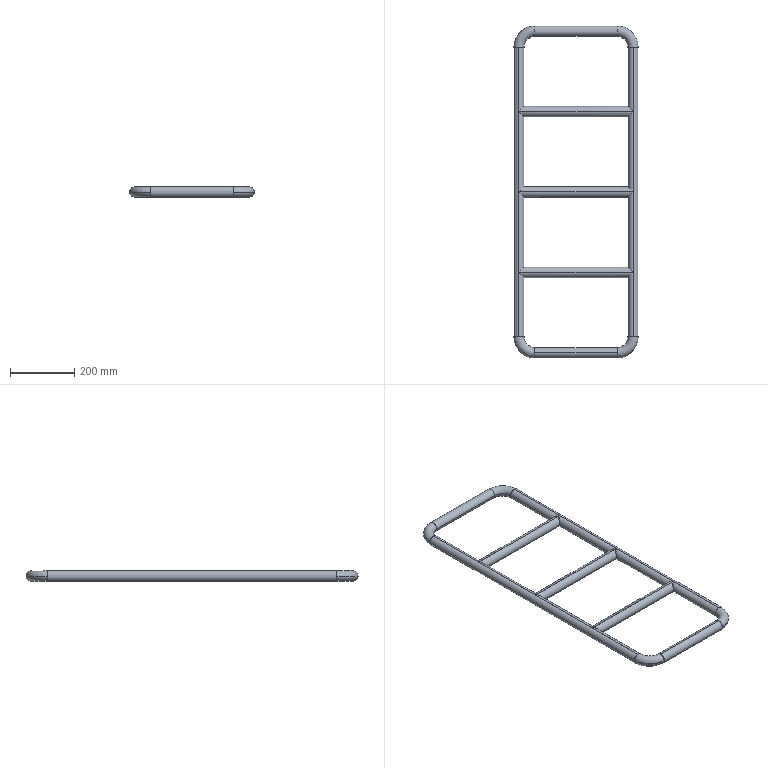Part | SolidWorks | features WeldMemberFeat 1, WeldmentFeature 1 | 11 solids | 66 faces | box 387 x 1032 x 32 mm | volume 682567 mm3 | cylinder 34 | plane 16 | torus 16 | commonest cylinder face diameters 32 x20 28 x14